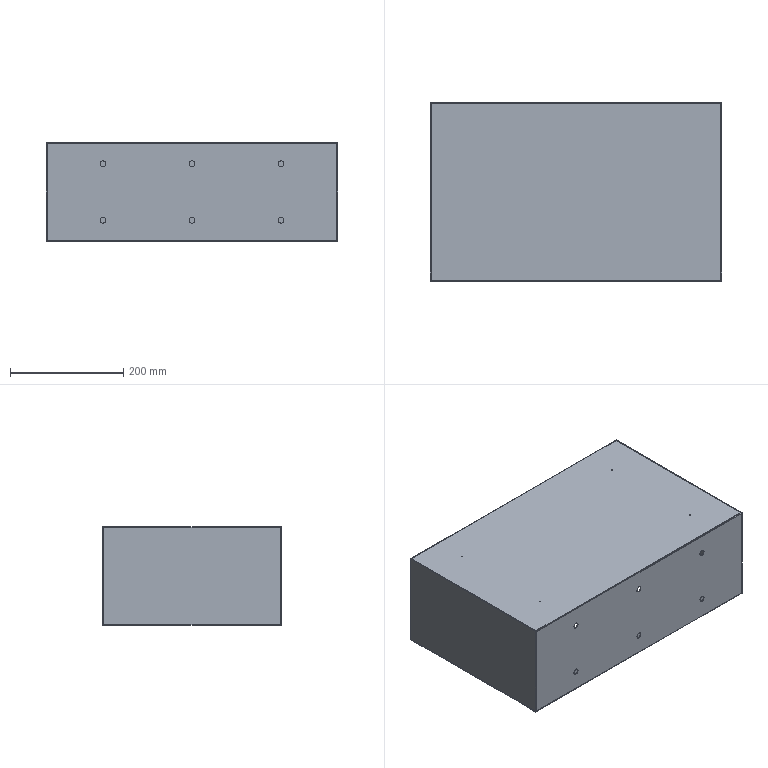Part | 3 solids | 246 faces | box 515 x 315 x 175 mm | volume 788956 mm3 | plane 162 | cylinder 84 | commonest cylinder face diameters 0.2 x14 3.2 x14 10 x12 16 x12 2 x8 5.2 x8